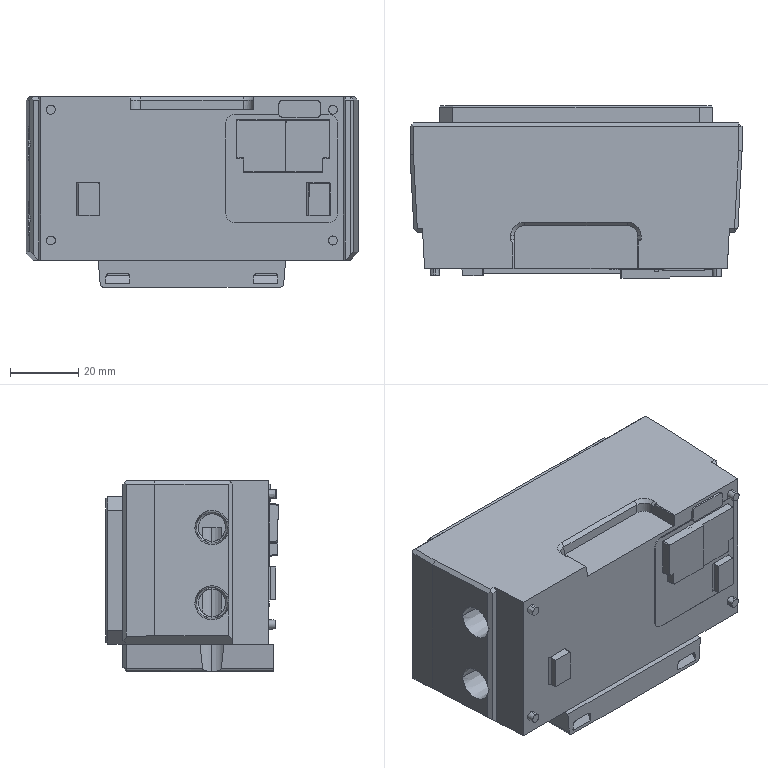Part | Creo | 1 solid | 355 faces | box 97 x 50.33 x 55.677 mm | volume 210136 mm3 | plane 164 | other 106 | cylinder 53 | cone 25 | spline 7 | commonest cylinder face diameters 8 x22 0.603 x8 2.01 x6 0.602 x5 10 x4 2.543 x2